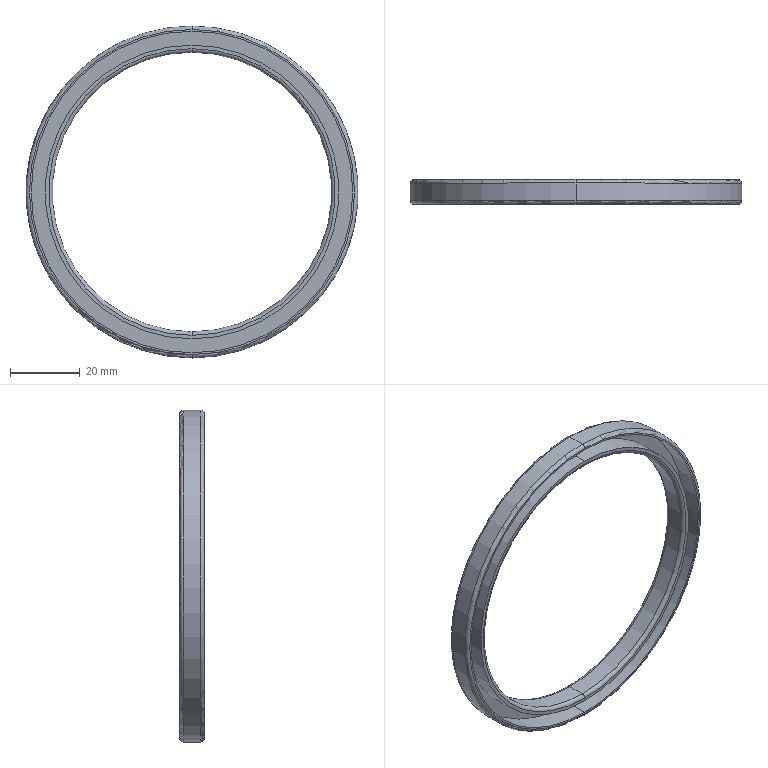Part | STEP file | 2026.6.15-Main Assembly图.sldasm-Part-123 | 1 solid | 82 faces | box 95 x 7 x 95 mm | volume 7521 mm3 | plane 40 | cylinder 34 | torus 8 | commonest cylinder face diameters 84.238 x13 90.837 x13 80 x2 84 x2 92 x2 95 x2